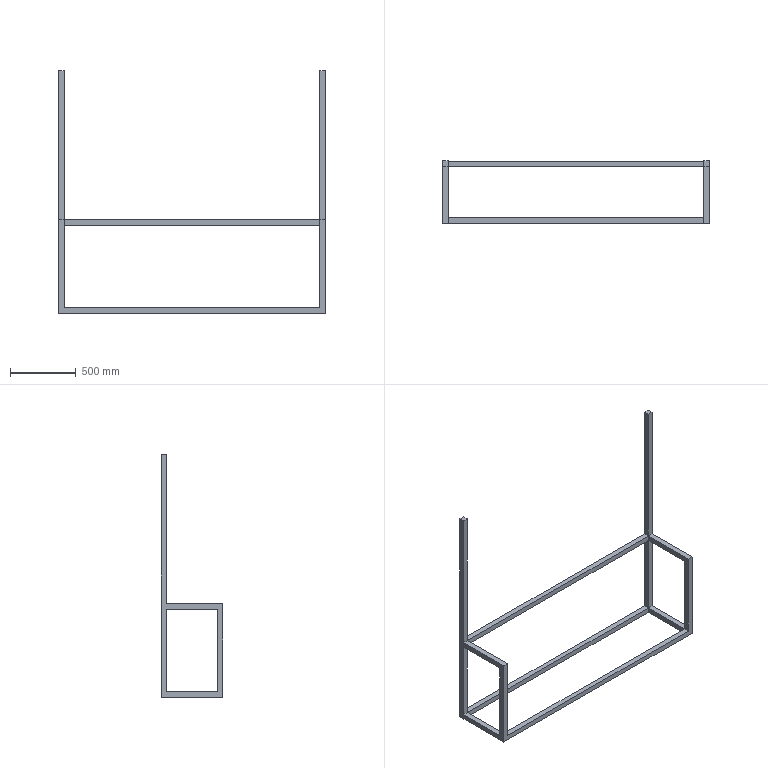Part | STEP file | Upper frame 2 | 1 solid | 34 faces | box 2022 x 470 x 1840 mm | volume 19970720 mm3 | plane 34